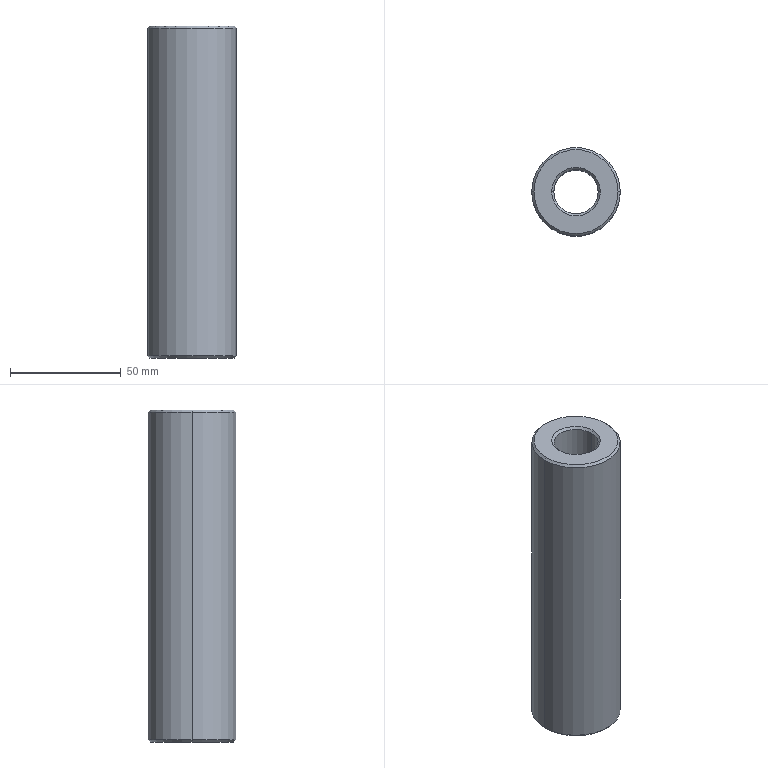Part | STEP file | BCC3 H17_2 | 1 solid | 14 faces | box 40 x 40 x 150 mm | volume 141183 mm3 | cone 8 | cylinder 4 | plane 2 | commonest cylinder face diameters 20 x2 40 x2
STEP:
#1=CARTESIAN_POINT('',(0.,0.,0.));
#2=DIRECTION('',(0.,0.,1.));
#3=DIRECTION('',(1.,0.,0.));
#4=AXIS2_PLACEMENT_3D('',#1,#2,#3);
#5=CARTESIAN_POINT('',(10.,0.,74.));
#6=VERTEX_POINT('',#5);
#7=CARTESIAN_POINT('',(11.,0.,75.));
#8=VERTEX_POINT('',#7);
#9=CARTESIAN_POINT('',(10.,0.,74.));
#10=DIRECTION('',(0.7071,0.,0.7071));
#11=VECTOR('',#10,1.);
#12=LINE('',#9,#11);
#13=CARTESIAN_POINT('',(0.,0.,74.));
#14=DIRECTION('',(0.,0.,1.));
#15=DIRECTION('',(1.,0.,0.));
#16=AXIS2_PLACEMENT_3D('',#13,#14,#15);
#17=CONICAL_SURFACE('',#16,10.,0.7854);
#18=CARTESIAN_POINT('',(6.283,0.));
#19=DIRECTION('',(0.,1.));
#20=VECTOR('',#19,1.);
#21=LINE('',#18,#20);
#22=(GEOMETRIC_REPRESENTATION_CONTEXT(2)PARAMETRIC_REPRESENTATION_CONTEXT()REPRESENTATION_CONTEXT('',''));
#23=DEFINITIONAL_REPRESENTATION('',(#21),#22);
#24=PCURVE('',#17,#23);
#25=CARTESIAN_POINT('',(0.,0.,74.));
#26=DIRECTION('',(0.,0.,1.));
#27=DIRECTION('',(1.,0.,0.));
#28=AXIS2_PLACEMENT_3D('',#25,#26,#27);
#29=CONICAL_SURFACE('',#28,10.,0.7854);
#30=CARTESIAN_POINT('',(0.,0.));
#31=DIRECTION('',(0.,1.));
#32=VECTOR('',#31,1.);
#33=LINE('',#30,#32);
#34=(GEOMETRIC_REPRESENTATION_CONTEXT(2)PARAMETRIC_REPRESENTATION_CONTEXT()REPRESENTATION_CONTEXT('',''));
#35=DEFINITIONAL_REPRESENTATION('',(#33),#34);
#36=PCURVE('',#29,#35);
#37=SURFACE_CURVE('',#12,(#24,#36),.PCURVE_S1.);
#38=EDGE_CURVE('',#6,#8,#37,.T.);
#39=ORIENTED_EDGE('',*,*,#38,.T.);
#40=CARTESIAN_POINT('',(-11.,0.,75.));
#41=VERTEX_POINT('',#40);
#42=CARTESIAN_POINT('',(0.,0.,75.));
#43=DIRECTION('',(0.,0.,-1.));
#44=DIRECTION('',(1.,0.,0.));
#45=AXIS2_PLACEMENT_3D('',#42,#43,#44);
#46=CIRCLE('',#45,11.);
#47=CARTESIAN_POINT('',(6.283,1.));
#48=DIRECTION('',(-1.,0.));
#49=VECTOR('',#48,1.);
#50=LINE('',#47,#49);
#51=(GEOMETRIC_REPRESENTATION_CONTEXT(2)PARAMETRIC_REPRESENTATION_CONTEXT()REPRESENTATION_CONTEXT('',''));
#52=DEFINITIONAL_REPRESENTATION('',(#50),#51);
#53=PCURVE('',#17,#52);
#54=CARTESIAN_POINT('',(0.,0.,75.));
#55=DIRECTION('',(0.,0.,1.));
#56=DIRECTION('',(1.,0.,0.));
#57=AXIS2_PLACEMENT_3D('',#54,#55,#56);
#58=PLANE('',#57);
#59=CARTESIAN_POINT('',(11.,0.));
#60=CARTESIAN_POINT('',(11.,-19.053));
#61=CARTESIAN_POINT('',(-5.5,-9.526));
#62=CARTESIAN_POINT('',(-22.,0.));
#63=CARTESIAN_POINT('',(-5.5,9.526));
#64=CARTESIAN_POINT('',(11.,19.053));
#65=CARTESIAN_POINT('',(11.,0.));
#66=(BOUNDED_CURVE()B_SPLINE_CURVE(2,(#59,#60,#61,#62,#63,#64,#65),.UNSPECIFIED.,.T.,.F.)B_SPLINE_CURVE_WITH_KNOTS((1,2,2,2,2,1),(-2.094,0.,2.094,4.189,6.283,8.378),.UNSPECIFIED.)CURVE()GEOMETRIC_REPRESENTATION_ITEM()RATIONAL_B_SPLINE_CURVE((1.,0.5,1.,0.5,1.,0.5,1.))REPRESENTATION_ITEM(''));
#67=(GEOMETRIC_REPRESENTATION_CONTEXT(2)PARAMETRIC_REPRESENTATION_CONTEXT()REPRESENTATION_CONTEXT('',''));
#68=DEFINITIONAL_REPRESENTATION('',(#66),#67);
#69=PCURVE('',#58,#68);
#70=SURFACE_CURVE('',#46,(#53,#69),.PCURVE_S1.);
#71=EDGE_CURVE('',#8,#41,#70,.T.);
#72=ORIENTED_EDGE('',*,*,#71,.T.);
#73=CARTESIAN_POINT('',(-10.,0.,74.));
#74=VERTEX_POINT('',#73);
#75=CARTESIAN_POINT('',(-10.,0.,74.));
#76=DIRECTION('',(-0.7071,0.,0.7071));
#77=VECTOR('',#76,1.);
#78=LINE('',#75,#77);
#79=CARTESIAN_POINT('',(3.142,0.));
#80=DIRECTION('',(0.,1.));
#81=VECTOR('',#80,1.);
#82=LINE('',#79,#81);
#83=(GEOMETRIC_REPRESENTATION_CONTEXT(2)PARAMETRIC_REPRESENTATION_CONTEXT()REPRESENTATION_CONTEXT('',''));
#84=DEFINITIONAL_REPRESENTATION('',(#82),#83);
#85=PCURVE('',#17,#84);
#86=CARTESIAN_POINT('',(3.142,0.));
#87=DIRECTION('',(0.,1.));
#88=VECTOR('',#87,1.);
#89=LINE('',#86,#88);
#90=(GEOMETRIC_REPRESENTATION_CONTEXT(2)PARAMETRIC_REPRESENTATION_CONTEXT()REPRESENTATION_CONTEXT('',''));
#91=DEFINITIONAL_REPRESENTATION('',(#89),#90);
#92=PCURVE('',#29,#91);
#93=SURFACE_CURVE('',#78,(#85,#92),.PCURVE_S1.);
#94=EDGE_CURVE('',#74,#41,#93,.T.);
#95=ORIENTED_EDGE('',*,*,#94,.F.);
#96=CARTESIAN_POINT('',(0.,0.,74.));
#97=DIRECTION('',(0.,0.,1.));
#98=DIRECTION('',(1.,0.,0.));
#99=AXIS2_PLACEMENT_3D('',#96,#97,#98);
#100=CIRCLE('',#99,10.);
#101=CARTESIAN_POINT('',(0.,0.));
#102=DIRECTION('',(1.,0.));
#103=VECTOR('',#102,1.);
#104=LINE('',#101,#103);
#105=(GEOMETRIC_REPRESENTATION_CONTEXT(2)PARAMETRIC_REPRESENTATION_CONTEXT()REPRESENTATION_CONTEXT('',''));
#106=DEFINITIONAL_REPRESENTATION('',(#104),#105);
#107=PCURVE('',#17,#106);
#108=CARTESIAN_POINT('',(0.,0.,75.));
#109=DIRECTION('',(0.,0.,-1.));
#110=DIRECTION('',(-1.,0.,0.));
#111=AXIS2_PLACEMENT_3D('',#108,#109,#110);
#112=CYLINDRICAL_SURFACE('',#111,10.);
#113=CARTESIAN_POINT('',(9.425,1.));
#114=DIRECTION('',(-1.,0.));
#115=VECTOR('',#114,1.);
#116=LINE('',#113,#115);
#117=(GEOMETRIC_REPRESENTATION_CONTEXT(2)PARAMETRIC_REPRESENTATION_CONTEXT()REPRESENTATION_CONTEXT('',''));
#118=DEFINITIONAL_REPRESENTATION('',(#116),#117);
#119=PCURVE('',#112,#118);
#120=SURFACE_CURVE('',#100,(#107,#119),.PCURVE_S1.);
#121=EDGE_CURVE('',#74,#6,#120,.T.);
#122=ORIENTED_EDGE('',*,*,#121,.T.);
#123=EDGE_LOOP('',(#39,#72,#95,#122));
#124=FACE_BOUND('',#123,.F.);
#125=ADVANCED_FACE('',(#124),#17,.F.);
#126=CARTESIAN_POINT('',(19.,0.,75.));
#127=VERTEX_POINT('',#126);
#128=CARTESIAN_POINT('',(-19.,0.,75.));
#129=VERTEX_POINT('',#128);
#130=CARTESIAN_POINT('',(0.,0.,75.));
#131=DIRECTION('',(0.,0.,1.));
#132=DIRECTION('',(1.,0.,0.));
#133=AXIS2_PLACEMENT_3D('',#130,#131,#132);
#134=CIRCLE('',#133,19.);
#135=CARTESIAN_POINT('',(0.,0.,75.));
#136=DIRECTION('',(0.,0.,-1.));
#137=DIRECTION('',(-1.,0.,0.));
#138=AXIS2_PLACEMENT_3D('',#135,#136,#137);
#139=CONICAL_SURFACE('',#138,19.,0.7854);
#140=CARTESIAN_POINT('',(3.142,0.));
#141=DIRECTION('',(-1.,0.));
#142=VECTOR('',#141,1.);
#143=LINE('',#140,#142);
#144=(GEOMETRIC_REPRESENTATION_CONTEXT(2)PARAMETRIC_REPRESENTATION_CONTEXT()REPRESENTATION_CONTEXT('',''));
#145=DEFINITIONAL_REPRESENTATION('',(#143),#144);
#146=PCURVE('',#139,#145);
#147=CARTESIAN_POINT('',(0.,0.));
#148=DIRECTION('',(1.,0.));
#149=AXIS2_PLACEMENT_2D('',#147,#148);
#150=CIRCLE('',#149,19.);
#151=(GEOMETRIC_REPRESENTATION_CONTEXT(2)PARAMETRIC_REPRESENTATION_CONTEXT()REPRESENTATION_CONTEXT('',''));
#152=DEFINITIONAL_REPRESENTATION('',(#150),#151);
#153=PCURVE('',#58,#152);
#154=SURFACE_CURVE('',#134,(#146,#153),.PCURVE_S1.);
#155=EDGE_CURVE('',#127,#129,#154,.T.);
#156=ORIENTED_EDGE('',*,*,#155,.F.);
#157=CARTESIAN_POINT('',(20.,0.,74.));
#158=VERTEX_POINT('',#157);
#159=CARTESIAN_POINT('',(19.,0.,75.));
#160=DIRECTION('',(0.7071,0.,-0.7071));
#161=VECTOR('',#160,1.);
#162=LINE('',#159,#161);
#163=CARTESIAN_POINT('',(3.142,0.));
#164=DIRECTION('',(0.,1.));
#165=VECTOR('',#164,1.);
#166=LINE('',#163,#165);
#167=(GEOMETRIC_REPRESENTATION_CONTEXT(2)PARAMETRIC_REPRESENTATION_CONTEXT()REPRESENTATION_CONTEXT('',''));
#168=DEFINITIONAL_REPRESENTATION('',(#166),#167);
#169=PCURVE('',#139,#168);
#170=CARTESIAN_POINT('',(0.,0.,75.));
#171=DIRECTION('',(0.,0.,-1.));
#172=DIRECTION('',(-1.,0.,0.));
#173=AXIS2_PLACEMENT_3D('',#170,#171,#172);
#174=CONICAL_SURFACE('',#173,19.,0.7854);
#175=CARTESIAN_POINT('',(3.142,0.));
#176=DIRECTION('',(0.,1.));
#177=VECTOR('',#176,1.);
#178=LINE('',#175,#177);
#179=(GEOMETRIC_REPRESENTATION_CONTEXT(2)PARAMETRIC_REPRESENTATION_CONTEXT()REPRESENTATION_CONTEXT('',''));
#180=DEFINITIONAL_REPRESENTATION('',(#178),#179);
#181=PCURVE('',#174,#180);
#182=SURFACE_CURVE('',#162,(#169,#181),.PCURVE_S1.);
#183=EDGE_CURVE('',#127,#158,#182,.T.);
#184=ORIENTED_EDGE('',*,*,#183,.T.);
#185=CARTESIAN_POINT('',(-20.,0.,74.));
#186=VERTEX_POINT('',#185);
#187=CARTESIAN_POINT('',(0.,0.,74.));
#188=DIRECTION('',(0.,0.,-1.));
#189=DIRECTION('',(1.,0.,0.));
#190=AXIS2_PLACEMENT_3D('',#187,#188,#189);
#191=CIRCLE('',#190,20.);
#192=CARTESIAN_POINT('',(-3.142,1.));
#193=DIRECTION('',(1.,0.));
#194=VECTOR('',#193,1.);
#195=LINE('',#192,#194);
#196=(GEOMETRIC_REPRESENTATION_CONTEXT(2)PARAMETRIC_REPRESENTATION_CONTEXT()REPRESENTATION_CONTEXT('',''));
#197=DEFINITIONAL_REPRESENTATION('',(#195),#196);
#198=PCURVE('',#139,#197);
#199=CARTESIAN_POINT('',(0.,0.,75.));
#200=DIRECTION('',(0.,0.,-1.));
#201=DIRECTION('',(-1.,0.,0.));
#202=AXIS2_PLACEMENT_3D('',#199,#200,#201);
#203=CYLINDRICAL_SURFACE('',#202,20.);
#204=CARTESIAN_POINT('',(-3.142,1.));
#205=DIRECTION('',(1.,0.));
#206=VECTOR('',#205,1.);
#207=LINE('',#204,#206);
#208=(GEOMETRIC_REPRESENTATION_CONTEXT(2)PARAMETRIC_REPRESENTATION_CONTEXT()REPRESENTATION_CONTEXT('',''));
#209=DEFINITIONAL_REPRESENTATION('',(#207),#208);
#210=PCURVE('',#203,#209);
#211=SURFACE_CURVE('',#191,(#198,#210),.PCURVE_S1.);
#212=EDGE_CURVE('',#186,#158,#211,.T.);
#213=ORIENTED_EDGE('',*,*,#212,.F.);
#214=CARTESIAN_POINT('',(-19.,0.,75.));
#215=DIRECTION('',(-0.7071,0.,-0.7071));
#216=VECTOR('',#215,1.);
#217=LINE('',#214,#216);
#218=CARTESIAN_POINT('',(0.,0.));
#219=DIRECTION('',(0.,1.));
#220=VECTOR('',#219,1.);
#221=LINE('',#218,#220);
#222=(GEOMETRIC_REPRESENTATION_CONTEXT(2)PARAMETRIC_REPRESENTATION_CONTEXT()REPRESENTATION_CONTEXT('',''));
#223=DEFINITIONAL_REPRESENTATION('',(#221),#222);
#224=PCURVE('',#139,#223);
#225=CARTESIAN_POINT('',(6.283,0.));
#226=DIRECTION('',(0.,1.));
#227=VECTOR('',#226,1.);
#228=LINE('',#225,#227);
#229=(GEOMETRIC_REPRESENTATION_CONTEXT(2)PARAMETRIC_REPRESENTATION_CONTEXT()REPRESENTATION_CONTEXT('',''));
#230=DEFINITIONAL_REPRESENTATION('',(#228),#229);
#231=PCURVE('',#174,#230);
#232=SURFACE_CURVE('',#217,(#224,#231),.PCURVE_S1.);
#233=EDGE_CURVE('',#129,#186,#232,.T.);
#234=ORIENTED_EDGE('',*,*,#233,.F.);
#235=EDGE_LOOP('',(#156,#184,#213,#234));
#236=FACE_BOUND('',#235,.T.);
#237=ADVANCED_FACE('',(#236),#139,.T.);
#238=CARTESIAN_POINT('',(-19.,0.,-75.));
#239=VERTEX_POINT('',#238);
#240=CARTESIAN_POINT('',(19.,0.,-75.));
#241=VERTEX_POINT('',#240);
#242=CARTESIAN_POINT('',(0.,0.,-75.));
#243=DIRECTION('',(0.,0.,-1.));
#244=DIRECTION('',(1.,0.,0.));
#245=AXIS2_PLACEMENT_3D('',#242,#243,#244);
#246=CIRCLE('',#245,19.);
#247=CARTESIAN_POINT('',(0.,0.,-74.));
#248=DIRECTION('',(0.,0.,1.));
#249=DIRECTION('',(1.,0.,0.));
#250=AXIS2_PLACEMENT_3D('',#247,#248,#249);
#251=CONICAL_SURFACE('',#250,20.,0.7854);
#252=CARTESIAN_POINT('',(6.283,-1.));
#253=DIRECTION('',(-1.,0.));
#254=VECTOR('',#253,1.);
#255=LINE('',#252,#254);
#256=(GEOMETRIC_REPRESENTATION_CONTEXT(2)PARAMETRIC_REPRESENTATION_CONTEXT()REPRESENTATION_CONTEXT('',''));
#257=DEFINITIONAL_REPRESENTATION('',(#255),#256);
#258=PCURVE('',#251,#257);
#259=CARTESIAN_POINT('',(0.,0.,-75.));
#260=DIRECTION('',(0.,0.,1.));
#261=DIRECTION('',(1.,0.,0.));
#262=AXIS2_PLACEMENT_3D('',#259,#260,#261);
#263=PLANE('',#262);
#264=CARTESIAN_POINT('',(19.,0.));
#265=CARTESIAN_POINT('',(19.,-32.909));
#266=CARTESIAN_POINT('',(-9.5,-16.454));
#267=CARTESIAN_POINT('',(-38.,0.));
#268=CARTESIAN_POINT('',(-9.5,16.454));
#269=CARTESIAN_POINT('',(19.,32.909));
#270=CARTESIAN_POINT('',(19.,0.));
#271=(BOUNDED_CURVE()B_SPLINE_CURVE(2,(#264,#265,#266,#267,#268,#269,#270),.UNSPECIFIED.,.T.,.F.)B_SPLINE_CURVE_WITH_KNOTS((1,2,2,2,2,1),(-2.094,0.,2.094,4.189,6.283,8.378),.UNSPECIFIED.)CURVE()GEOMETRIC_REPRESENTATION_ITEM()RATIONAL_B_SPLINE_CURVE((1.,0.5,1.,0.5,1.,0.5,1.))REPRESENTATION_ITEM(''));
#272=(GEOMETRIC_REPRESENTATION_CONTEXT(2)PARAMETRIC_REPRESENTATION_CONTEXT()REPRESENTATION_CONTEXT('',''));
#273=DEFINITIONAL_REPRESENTATION('',(#271),#272);
#274=PCURVE('',#263,#273);
#275=SURFACE_CURVE('',#246,(#258,#274),.PCURVE_S1.);
#276=EDGE_CURVE('',#239,#241,#275,.T.);
#277=ORIENTED_EDGE('',*,*,#276,.F.);
#278=CARTESIAN_POINT('',(-20.,0.,-74.));
#279=VERTEX_POINT('',#278);
#280=CARTESIAN_POINT('',(-20.,0.,-74.));
#281=DIRECTION('',(-0.7071,0.,0.7071));
#282=VECTOR('',#281,1.);
#283=LINE('',#280,#282);
#284=CARTESIAN_POINT('',(3.142,0.));
#285=DIRECTION('',(0.,1.));
#286=VECTOR('',#285,1.);
#287=LINE('',#284,#286);
#288=(GEOMETRIC_REPRESENTATION_CONTEXT(2)PARAMETRIC_REPRESENTATION_CONTEXT()REPRESENTATION_CONTEXT('',''));
#289=DEFINITIONAL_REPRESENTATION('',(#287),#288);
#290=PCURVE('',#251,#289);
#291=CARTESIAN_POINT('',(0.,0.,-74.));
#292=DIRECTION('',(0.,0.,1.));
#293=DIRECTION('',(1.,0.,0.));
#294=AXIS2_PLACEMENT_3D('',#291,#292,#293);
#295=CONICAL_SURFACE('',#294,20.,0.7854);
#296=CARTESIAN_POINT('',(3.142,0.));
#297=DIRECTION('',(0.,1.));
#298=VECTOR('',#297,1.);
#299=LINE('',#296,#298);
#300=(GEOMETRIC_REPRESENTATION_CONTEXT(2)PARAMETRIC_REPRESENTATION_CONTEXT()REPRESENTATION_CONTEXT('',''));
#301=DEFINITIONAL_REPRESENTATION('',(#299),#300);
#302=PCURVE('',#295,#301);
#303=SURFACE_CURVE('',#283,(#290,#302),.PCURVE_S1.);
#304=EDGE_CURVE('',#239,#279,#303,.T.);
#305=ORIENTED_EDGE('',*,*,#304,.T.);
#306=CARTESIAN_POINT('',(20.,0.,-74.));
#307=VERTEX_POINT('',#306);
#308=CARTESIAN_POINT('',(0.,0.,-74.));
#309=DIRECTION('',(0.,0.,1.));
#310=DIRECTION('',(1.,0.,0.));
#311=AXIS2_PLACEMENT_3D('',#308,#309,#310);
#312=CIRCLE('',#311,20.);
#313=CARTESIAN_POINT('',(0.,0.));
#314=DIRECTION('',(1.,0.));
#315=VECTOR('',#314,1.);
#316=LINE('',#313,#315);
#317=(GEOMETRIC_REPRESENTATION_CONTEXT(2)PARAMETRIC_REPRESENTATION_CONTEXT()REPRESENTATION_CONTEXT('',''));
#318=DEFINITIONAL_REPRESENTATION('',(#316),#317);
#319=PCURVE('',#251,#318);
#320=CARTESIAN_POINT('',(3.142,149.));
#321=DIRECTION('',(-1.,0.));
#322=VECTOR('',#321,1.);
#323=LINE('',#320,#322);
#324=(GEOMETRIC_REPRESENTATION_CONTEXT(2)PARAMETRIC_REPRESENTATION_CONTEXT()REPRESENTATION_CONTEXT('',''));
#325=DEFINITIONAL_REPRESENTATION('',(#323),#324);
#326=PCURVE('',#203,#325);
#327=SURFACE_CURVE('',#312,(#319,#326),.PCURVE_S1.);
#328=EDGE_CURVE('',#307,#279,#327,.T.);
#329=ORIENTED_EDGE('',*,*,#328,.F.);
#330=CARTESIAN_POINT('',(20.,0.,-74.));
#331=DIRECTION('',(0.7071,0.,0.7071));
#332=VECTOR('',#331,1.);
#333=LINE('',#330,#332);
#334=CARTESIAN_POINT('',(0.,0.));
#335=DIRECTION('',(0.,1.));
#336=VECTOR('',#335,1.);
#337=LINE('',#334,#336);
#338=(GEOMETRIC_REPRESENTATION_CONTEXT(2)PARAMETRIC_REPRESENTATION_CONTEXT()REPRESENTATION_CONTEXT('',''));
#339=DEFINITIONAL_REPRESENTATION('',(#337),#338);
#340=PCURVE('',#251,#339);
#341=CARTESIAN_POINT('',(6.283,0.));
#342=DIRECTION('',(0.,1.));
#343=VECTOR('',#342,1.);
#344=LINE('',#341,#343);
#345=(GEOMETRIC_REPRESENTATION_CONTEXT(2)PARAMETRIC_REPRESENTATION_CONTEXT()REPRESENTATION_CONTEXT('',''));
#346=DEFINITIONAL_REPRESENTATION('',(#344),#345);
#347=PCURVE('',#295,#346);
#348=SURFACE_CURVE('',#333,(#340,#347),.PCURVE_S1.);
#349=EDGE_CURVE('',#241,#307,#348,.T.);
#350=ORIENTED_EDGE('',*,*,#349,.F.);
#351=EDGE_LOOP('',(#277,#305,#329,#350));
#352=FACE_BOUND('',#351,.T.);
#353=ADVANCED_FACE('',(#352),#251,.T.);
#354=CARTESIAN_POINT('',(-10.,0.,-74.));
#355=VERTEX_POINT('',#354);
#356=CARTESIAN_POINT('',(-11.,0.,-75.));
#357=VERTEX_POINT('',#356);
#358=CARTESIAN_POINT('',(-11.,0.,-75.));
#359=DIRECTION('',(-0.7071,0.,-0.7071));
#360=VECTOR('',#359,1.);
#361=LINE('',#358,#360);
#362=CARTESIAN_POINT('',(0.,0.,-75.));
#363=DIRECTION('',(0.,0.,-1.));
#364=DIRECTION('',(-1.,0.,0.));
#365=AXIS2_PLACEMENT_3D('',#362,#363,#364);
#366=CONICAL_SURFACE('',#365,11.,0.7854);
#367=CARTESIAN_POINT('',(6.283,0.));
#368=DIRECTION('',(0.,1.));
#369=VECTOR('',#368,1.);
#370=LINE('',#367,#369);
#371=(GEOMETRIC_REPRESENTATION_CONTEXT(2)PARAMETRIC_REPRESENTATION_CONTEXT()REPRESENTATION_CONTEXT('',''));
#372=DEFINITIONAL_REPRESENTATION('',(#370),#371);
#373=PCURVE('',#366,#372);
#374=CARTESIAN_POINT('',(0.,0.,-75.));
#375=DIRECTION('',(0.,0.,-1.));
#376=DIRECTION('',(-1.,0.,0.));
#377=AXIS2_PLACEMENT_3D('',#374,#375,#376);
#378=CONICAL_SURFACE('',#377,11.,0.7854);
#379=CARTESIAN_POINT('',(0.,0.));
#380=DIRECTION('',(0.,1.));
#381=VECTOR('',#380,1.);
#382=LINE('',#379,#381);
#383=(GEOMETRIC_REPRESENTATION_CONTEXT(2)PARAMETRIC_REPRESENTATION_CONTEXT()REPRESENTATION_CONTEXT('',''));
#384=DEFINITIONAL_REPRESENTATION('',(#382),#383);
#385=PCURVE('',#378,#384);
#386=SURFACE_CURVE('',#361,(#373,#385),.PCURVE_S1.);
#387=EDGE_CURVE('',#355,#357,#386,.T.);
#388=ORIENTED_EDGE('',*,*,#387,.T.);
#389=CARTESIAN_POINT('',(11.,0.,-75.));
#390=VERTEX_POINT('',#389);
#391=CARTESIAN_POINT('',(0.,0.,-75.));
#392=DIRECTION('',(0.,0.,1.));
#393=DIRECTION('',(1.,0.,0.));
#394=AXIS2_PLACEMENT_3D('',#391,#392,#393);
#395=CIRCLE('',#394,11.);
#396=CARTESIAN_POINT('',(9.425,0.));
#397=DIRECTION('',(-1.,0.));
#398=VECTOR('',#397,1.);
#399=LINE('',#396,#398);
#400=(GEOMETRIC_REPRESENTATION_CONTEXT(2)PARAMETRIC_REPRESENTATION_CONTEXT()REPRESENTATION_CONTEXT('',''));
#401=DEFINITIONAL_REPRESENTATION('',(#399),#400);
#402=PCURVE('',#366,#401);
#403=CARTESIAN_POINT('',(0.,0.));
#404=DIRECTION('',(1.,0.));
#405=AXIS2_PLACEMENT_2D('',#403,#404);
#406=CIRCLE('',#405,11.);
#407=(GEOMETRIC_REPRESENTATION_CONTEXT(2)PARAMETRIC_REPRESENTATION_CONTEXT()REPRESENTATION_CONTEXT('',''));
#408=DEFINITIONAL_REPRESENTATION('',(#406),#407);
#409=PCURVE('',#263,#408);
#410=SURFACE_CURVE('',#395,(#402,#409),.PCURVE_S1.);
#411=EDGE_CURVE('',#357,#390,#410,.T.);
#412=ORIENTED_EDGE('',*,*,#411,.T.);
#413=CARTESIAN_POINT('',(10.,0.,-74.));
#414=VERTEX_POINT('',#413);
#415=CARTESIAN_POINT('',(11.,0.,-75.));
#416=DIRECTION('',(0.7071,0.,-0.7071));
#417=VECTOR('',#416,1.);
#418=LINE('',#415,#417);
#419=CARTESIAN_POINT('',(3.142,0.));
#420=DIRECTION('',(0.,1.));
#421=VECTOR('',#420,1.);
#422=LINE('',#419,#421);
#423=(GEOMETRIC_REPRESENTATION_CONTEXT(2)PARAMETRIC_REPRESENTATION_CONTEXT()REPRESENTATION_CONTEXT('',''));
#424=DEFINITIONAL_REPRESENTATION('',(#422),#423);
#425=PCURVE('',#366,#424);
#426=CARTESIAN_POINT('',(3.142,0.));
#427=DIRECTION('',(0.,1.));
#428=VECTOR('',#427,1.);
#429=LINE('',#426,#428);
#430=(GEOMETRIC_REPRESENTATION_CONTEXT(2)PARAMETRIC_REPRESENTATION_CONTEXT()REPRESENTATION_CONTEXT('',''));
#431=DEFINITIONAL_REPRESENTATION('',(#429),#430);
#432=PCURVE('',#378,#431);
#433=SURFACE_CURVE('',#418,(#425,#432),.PCURVE_S1.);
#434=EDGE_CURVE('',#414,#390,#433,.T.);
#435=ORIENTED_EDGE('',*,*,#434,.F.);
#436=CARTESIAN_POINT('',(0.,0.,-74.));
#437=DIRECTION('',(0.,0.,-1.));
#438=DIRECTION('',(1.,0.,0.));
#439=AXIS2_PLACEMENT_3D('',#436,#437,#438);
#440=CIRCLE('',#439,10.);
#441=CARTESIAN_POINT('',(3.142,-1.));
#442=DIRECTION('',(1.,0.));
#443=VECTOR('',#442,1.);
#444=LINE('',#441,#443);
#445=(GEOMETRIC_REPRESENTATION_CONTEXT(2)PARAMETRIC_REPRESENTATION_CONTEXT()REPRESENTATION_CONTEXT('',''));
#446=DEFINITIONAL_REPRESENTATION('',(#444),#445);
#447=PCURVE('',#366,#446);
#448=CARTESIAN_POINT('',(3.142,149.));
#449=DIRECTION('',(1.,0.));
#450=VECTOR('',#449,1.);
#451=LINE('',#448,#450);
#452=(GEOMETRIC_REPRESENTATION_CONTEXT(2)PARAMETRIC_REPRESENTATION_CONTEXT()REPRESENTATION_CONTEXT('',''));
#453=DEFINITIONAL_REPRESENTATION('',(#451),#452);
#454=PCURVE('',#112,#453);
#455=SURFACE_CURVE('',#440,(#447,#454),.PCURVE_S1.);
#456=EDGE_CURVE('',#414,#355,#455,.T.);
#457=ORIENTED_EDGE('',*,*,#456,.T.);
#458=EDGE_LOOP('',(#388,#412,#435,#457));
#459=FACE_BOUND('',#458,.F.);
#460=ADVANCED_FACE('',(#459),#366,.F.);
#461=CARTESIAN_POINT('',(-10.,0.,75.));
#462=DIRECTION('',(0.,0.,-1.));
#463=VECTOR('',#462,1.);
#464=LINE('',#461,#463);
#465=CARTESIAN_POINT('',(6.283,0.));
#466=DIRECTION('',(0.,1.));
#467=VECTOR('',#466,1.);
#468=LINE('',#465,#467);
#469=(GEOMETRIC_REPRESENTATION_CONTEXT(2)PARAMETRIC_REPRESENTATION_CONTEXT()REPRESENTATION_CONTEXT('',''));
#470=DEFINITIONAL_REPRESENTATION('',(#468),#469);
#471=PCURVE('',#112,#470);
#472=CARTESIAN_POINT('',(0.,0.,75.));
#473=DIRECTION('',(0.,0.,-1.));
#474=DIRECTION('',(-1.,0.,0.));
#475=AXIS2_PLACEMENT_3D('',#472,#473,#474);
#476=CYLINDRICAL_SURFACE('',#475,10.);
#477=CARTESIAN_POINT('',(0.,0.));
#478=DIRECTION('',(0.,1.));
#479=VECTOR('',#478,1.);
#480=LINE('',#477,#479);
#481=(GEOMETRIC_REPRESENTATION_CONTEXT(2)PARAMETRIC_REPRESENTATION_CONTEXT()REPRESENTATION_CONTEXT('',''));
#482=DEFINITIONAL_REPRESENTATION('',(#480),#481);
#483=PCURVE('',#476,#482);
#484=SURFACE_CURVE('',#464,(#471,#483),.PCURVE_S1.);
#485=EDGE_CURVE('',#74,#355,#484,.T.);
#486=ORIENTED_EDGE('',*,*,#485,.T.);
#487=ORIENTED_EDGE('',*,*,#456,.F.);
#488=CARTESIAN_POINT('',(10.,0.,75.));
#489=DIRECTION('',(0.,0.,-1.));
#490=VECTOR('',#489,1.);
#491=LINE('',#488,#490);
#492=CARTESIAN_POINT('',(3.142,0.));
#493=DIRECTION('',(0.,1.));
#494=VECTOR('',#493,1.);
#495=LINE('',#492,#494);
#496=(GEOMETRIC_REPRESENTATION_CONTEXT(2)PARAMETRIC_REPRESENTATION_CONTEXT()REPRESENTATION_CONTEXT('',''));
#497=DEFINITIONAL_REPRESENTATION('',(#495),#496);
#498=PCURVE('',#112,#497);
#499=CARTESIAN_POINT('',(3.142,0.));
#500=DIRECTION('',(0.,1.));
#501=VECTOR('',#500,1.);
#502=LINE('',#499,#501);
#503=(GEOMETRIC_REPRESENTATION_CONTEXT(2)PARAMETRIC_REPRESENTATION_CONTEXT()REPRESENTATION_CONTEXT('',''));
#504=DEFINITIONAL_REPRESENTATION('',(#502),#503);
#505=PCURVE('',#476,#504);
#506=SURFACE_CURVE('',#491,(#498,#505),.PCURVE_S1.);
#507=EDGE_CURVE('',#6,#414,#506,.T.);
#508=ORIENTED_EDGE('',*,*,#507,.F.);
#509=ORIENTED_EDGE('',*,*,#121,.F.);
#510=EDGE_LOOP('',(#486,#487,#508,#509));
#511=FACE_BOUND('',#510,.F.);
#512=ADVANCED_FACE('',(#511),#112,.F.);
#513=ORIENTED_EDGE('',*,*,#212,.T.);
#514=CARTESIAN_POINT('',(20.,0.,75.));
#515=DIRECTION('',(0.,0.,-1.));
#516=VECTOR('',#515,1.);
#517=LINE('',#514,#516);
#518=CARTESIAN_POINT('',(3.142,0.));
#519=DIRECTION('',(0.,1.));
#520=VECTOR('',#519,1.);
#521=LINE('',#518,#520);
#522=(GEOMETRIC_REPRESENTATION_CONTEXT(2)PARAMETRIC_REPRESENTATION_CONTEXT()REPRESENTATION_CONTEXT('',''));
#523=DEFINITIONAL_REPRESENTATION('',(#521),#522);
#524=PCURVE('',#203,#523);
#525=CARTESIAN_POINT('',(0.,0.,75.));
#526=DIRECTION('',(0.,0.,-1.));
#527=DIRECTION('',(-1.,0.,0.));
#528=AXIS2_PLACEMENT_3D('',#525,#526,#527);
#529=CYLINDRICAL_SURFACE('',#528,20.);
#530=CARTESIAN_POINT('',(3.142,0.));
#531=DIRECTION('',(0.,1.));
#532=VECTOR('',#531,1.);
#533=LINE('',#530,#532);
#534=(GEOMETRIC_REPRESENTATION_CONTEXT(2)PARAMETRIC_REPRESENTATION_CONTEXT()REPRESENTATION_CONTEXT('',''));
#535=DEFINITIONAL_REPRESENTATION('',(#533),#534);
#536=PCURVE('',#529,#535);
#537=SURFACE_CURVE('',#517,(#524,#536),.PCURVE_S1.);
#538=EDGE_CURVE('',#158,#307,#537,.T.);
#539=ORIENTED_EDGE('',*,*,#538,.T.);
#540=ORIENTED_EDGE('',*,*,#328,.T.);
#541=CARTESIAN_POINT('',(-20.,0.,75.));
#542=DIRECTION('',(0.,0.,-1.));
#543=VECTOR('',#542,1.);
#544=LINE('',#541,#543);
#545=CARTESIAN_POINT('',(0.,0.));
#546=DIRECTION('',(0.,1.));
#547=VECTOR('',#546,1.);
#548=LINE('',#545,#547);
#549=(GEOMETRIC_REPRESENTATION_CONTEXT(2)PARAMETRIC_REPRESENTATION_CONTEXT()REPRESENTATION_CONTEXT('',''));
#550=DEFINITIONAL_REPRESENTATION('',(#548),#549);
#551=PCURVE('',#203,#550);
#552=CARTESIAN_POINT('',(6.283,0.));
#553=DIRECTION('',(0.,1.));
#554=VECTOR('',#553,1.);
#555=LINE('',#552,#554);
#556=(GEOMETRIC_REPRESENTATION_CONTEXT(2)PARAMETRIC_REPRESENTATION_CONTEXT()REPRESENTATION_CONTEXT('',''));
#557=DEFINITIONAL_REPRESENTATION('',(#555),#556);
#558=PCURVE('',#529,#557);
#559=SURFACE_CURVE('',#544,(#551,#558),.PCURVE_S1.);
#560=EDGE_CURVE('',#186,#279,#559,.T.);
#561=ORIENTED_EDGE('',*,*,#560,.F.);
#562=EDGE_LOOP('',(#513,#539,#540,#561));
#563=FACE_BOUND('',#562,.T.);
#564=ADVANCED_FACE('',(#563),#203,.T.);
#565=CARTESIAN_POINT('',(0.,0.,75.));
#566=DIRECTION('',(0.,0.,1.));
#567=DIRECTION('',(1.,0.,0.));
#568=AXIS2_PLACEMENT_3D('',#565,#566,#567);
#569=CIRCLE('',#568,19.);
#570=CARTESIAN_POINT('',(0.,0.));
#571=DIRECTION('',(1.,0.));
#572=AXIS2_PLACEMENT_2D('',#570,#571);
#573=CIRCLE('',#572,19.);
#574=(GEOMETRIC_REPRESENTATION_CONTEXT(2)PARAMETRIC_REPRESENTATION_CONTEXT()REPRESENTATION_CONTEXT('',''));
#575=DEFINITIONAL_REPRESENTATION('',(#573),#574);
#576=PCURVE('',#58,#575);
#577=CARTESIAN_POINT('',(9.425,0.));
#578=DIRECTION('',(-1.,0.));
#579=VECTOR('',#578,1.);
#580=LINE('',#577,#579);
#581=(GEOMETRIC_REPRESENTATION_CONTEXT(2)PARAMETRIC_REPRESENTATION_CONTEXT()REPRESENTATION_CONTEXT('',''));
#582=DEFINITIONAL_REPRESENTATION('',(#580),#581);
#583=PCURVE('',#174,#582);
#584=SURFACE_CURVE('',#569,(#576,#583),.PCURVE_S1.);
#585=EDGE_CURVE('',#129,#127,#584,.T.);
#586=ORIENTED_EDGE('',*,*,#585,.T.);
#587=ORIENTED_EDGE('',*,*,#155,.T.);
#588=EDGE_LOOP('',(#586,#587));
#589=FACE_BOUND('',#588,.T.);
#590=ORIENTED_EDGE('',*,*,#71,.T.);
#591=CARTESIAN_POINT('',(0.,0.,75.));
#592=DIRECTION('',(0.,0.,-1.));
#593=DIRECTION('',(1.,0.,0.));
#594=AXIS2_PLACEMENT_3D('',#591,#592,#593);
#595=CIRCLE('',#594,11.);
#596=CARTESIAN_POINT('',(11.,0.));
#597=CARTESIAN_POINT('',(11.,-19.053));
#598=CARTESIAN_POINT('',(-5.5,-9.526));
#599=CARTESIAN_POINT('',(-22.,0.));
#600=CARTESIAN_POINT('',(-5.5,9.526));
#601=CARTESIAN_POINT('',(11.,19.053));
#602=CARTESIAN_POINT('',(11.,0.));
#603=(BOUNDED_CURVE()B_SPLINE_CURVE(2,(#596,#597,#598,#599,#600,#601,#602),.UNSPECIFIED.,.T.,.F.)B_SPLINE_CURVE_WITH_KNOTS((1,2,2,2,2,1),(-2.094,0.,2.094,4.189,6.283,8.378),.UNSPECIFIED.)CURVE()GEOMETRIC_REPRESENTATION_ITEM()RATIONAL_B_SPLINE_CURVE((1.,0.5,1.,0.5,1.,0.5,1.))REPRESENTATION_ITEM(''));
#604=(GEOMETRIC_REPRESENTATION_CONTEXT(2)PARAMETRIC_REPRESENTATION_CONTEXT()REPRESENTATION_CONTEXT('',''));
#605=DEFINITIONAL_REPRESENTATION('',(#603),#604);
#606=PCURVE('',#58,#605);
#607=CARTESIAN_POINT('',(6.283,1.));
#608=DIRECTION('',(-1.,0.));
#609=VECTOR('',#608,1.);
#610=LINE('',#607,#609);
#611=(GEOMETRIC_REPRESENTATION_CONTEXT(2)PARAMETRIC_REPRESENTATION_CONTEXT()REPRESENTATION_CONTEXT('',''));
#612=DEFINITIONAL_REPRESENTATION('',(#610),#611);
#613=PCURVE('',#29,#612);
#614=SURFACE_CURVE('',#595,(#606,#613),.PCURVE_S1.);
#615=EDGE_CURVE('',#41,#8,#614,.T.);
#616=ORIENTED_EDGE('',*,*,#615,.T.);
#617=EDGE_LOOP('',(#590,#616));
#618=FACE_BOUND('',#617,.T.);
#619=ADVANCED_FACE('',(#589,#618),#58,.T.);
#620=ORIENTED_EDGE('',*,*,#411,.T.);
#621=CARTESIAN_POINT('',(0.,0.,-75.));
#622=DIRECTION('',(0.,0.,1.));
#623=DIRECTION('',(1.,0.,0.));
#624=AXIS2_PLACEMENT_3D('',#621,#622,#623);
#625=CIRCLE('',#624,11.);
#626=CARTESIAN_POINT('',(0.,0.));
#627=DIRECTION('',(1.,0.));
#628=AXIS2_PLACEMENT_2D('',#626,#627);
#629=CIRCLE('',#628,11.);
#630=(GEOMETRIC_REPRESENTATION_CONTEXT(2)PARAMETRIC_REPRESENTATION_CONTEXT()REPRESENTATION_CONTEXT('',''));
#631=DEFINITIONAL_REPRESENTATION('',(#629),#630);
#632=PCURVE('',#263,#631);
#633=CARTESIAN_POINT('',(3.142,0.));
#634=DIRECTION('',(-1.,0.));
#635=VECTOR('',#634,1.);
#636=LINE('',#633,#635);
#637=(GEOMETRIC_REPRESENTATION_CONTEXT(2)PARAMETRIC_REPRESENTATION_CONTEXT()REPRESENTATION_CONTEXT('',''));
#638=DEFINITIONAL_REPRESENTATION('',(#636),#637);
#639=PCURVE('',#378,#638);
#640=SURFACE_CURVE('',#625,(#632,#639),.PCURVE_S1.);
#641=EDGE_CURVE('',#390,#357,#640,.T.);
#642=ORIENTED_EDGE('',*,*,#641,.T.);
#643=EDGE_LOOP('',(#620,#642));
#644=FACE_BOUND('',#643,.T.);
#645=CARTESIAN_POINT('',(0.,0.,-75.));
#646=DIRECTION('',(0.,0.,-1.));
#647=DIRECTION('',(1.,0.,0.));
#648=AXIS2_PLACEMENT_3D('',#645,#646,#647);
#649=CIRCLE('',#648,19.);
#650=CARTESIAN_POINT('',(19.,0.));
#651=CARTESIAN_POINT('',(19.,-32.909));
#652=CARTESIAN_POINT('',(-9.5,-16.454));
#653=CARTESIAN_POINT('',(-38.,0.));
#654=CARTESIAN_POINT('',(-9.5,16.454));
#655=CARTESIAN_POINT('',(19.,32.909));
#656=CARTESIAN_POINT('',(19.,0.));
#657=(BOUNDED_CURVE()B_SPLINE_CURVE(2,(#650,#651,#652,#653,#654,#655,#656),.UNSPECIFIED.,.T.,.F.)B_SPLINE_CURVE_WITH_KNOTS((1,2,2,2,2,1),(-2.094,0.,2.094,4.189,6.283,8.378),.UNSPECIFIED.)CURVE()GEOMETRIC_REPRESENTATION_ITEM()RATIONAL_B_SPLINE_CURVE((1.,0.5,1.,0.5,1.,0.5,1.))REPRESENTATION_ITEM(''));
#658=(GEOMETRIC_REPRESENTATION_CONTEXT(2)PARAMETRIC_REPRESENTATION_CONTEXT()REPRESENTATION_CONTEXT('',''));
#659=DEFINITIONAL_REPRESENTATION('',(#657),#658);
#660=PCURVE('',#263,#659);
#661=CARTESIAN_POINT('',(6.283,-1.));
#662=DIRECTION('',(-1.,0.));
#663=VECTOR('',#662,1.);
#664=LINE('',#661,#663);
#665=(GEOMETRIC_REPRESENTATION_CONTEXT(2)PARAMETRIC_REPRESENTATION_CONTEXT()REPRESENTATION_CONTEXT('',''));
#666=DEFINITIONAL_REPRESENTATION('',(#664),#665);
#667=PCURVE('',#295,#666);
#668=SURFACE_CURVE('',#649,(#660,#667),.PCURVE_S1.);
#669=EDGE_CURVE('',#241,#239,#668,.T.);
#670=ORIENTED_EDGE('',*,*,#669,.T.);
#671=ORIENTED_EDGE('',*,*,#276,.T.);
#672=EDGE_LOOP('',(#670,#671));
#673=FACE_BOUND('',#672,.T.);
#674=ADVANCED_FACE('',(#644,#673),#263,.F.);
#675=ORIENTED_EDGE('',*,*,#538,.F.);
#676=CARTESIAN_POINT('',(0.,0.,74.));
#677=DIRECTION('',(0.,0.,-1.));
#678=DIRECTION('',(1.,0.,0.));
#679=AXIS2_PLACEMENT_3D('',#676,#677,#678);
#680=CIRCLE('',#679,20.);
#681=CARTESIAN_POINT('',(3.142,1.));
#682=DIRECTION('',(1.,0.));
#683=VECTOR('',#682,1.);
#684=LINE('',#681,#683);
#685=(GEOMETRIC_REPRESENTATION_CONTEXT(2)PARAMETRIC_REPRESENTATION_CONTEXT()REPRESENTATION_CONTEXT('',''));
#686=DEFINITIONAL_REPRESENTATION('',(#684),#685);
#687=PCURVE('',#529,#686);
#688=CARTESIAN_POINT('',(3.142,1.));
#689=DIRECTION('',(1.,0.));
#690=VECTOR('',#689,1.);
#691=LINE('',#688,#690);
#692=(GEOMETRIC_REPRESENTATION_CONTEXT(2)PARAMETRIC_REPRESENTATION_CONTEXT()REPRESENTATION_CONTEXT('',''));
#693=DEFINITIONAL_REPRESENTATION('',(#691),#692);
#694=PCURVE('',#174,#693);
#695=SURFACE_CURVE('',#680,(#687,#694),.PCURVE_S1.);
#696=EDGE_CURVE('',#158,#186,#695,.T.);
#697=ORIENTED_EDGE('',*,*,#696,.T.);
#698=ORIENTED_EDGE('',*,*,#560,.T.);
#699=CARTESIAN_POINT('',(0.,0.,-74.));
#700=DIRECTION('',(0.,0.,1.));
#701=DIRECTION('',(1.,0.,0.));
#702=AXIS2_PLACEMENT_3D('',#699,#700,#701);
#703=CIRCLE('',#702,20.);
#704=CARTESIAN_POINT('',(9.425,149.));
#705=DIRECTION('',(-1.,0.));
#706=VECTOR('',#705,1.);
#707=LINE('',#704,#706);
#708=(GEOMETRIC_REPRESENTATION_CONTEXT(2)PARAMETRIC_REPRESENTATION_CONTEXT()REPRESENTATION_CONTEXT('',''));
#709=DEFINITIONAL_REPRESENTATION('',(#707),#708);
#710=PCURVE('',#529,#709);
#711=CARTESIAN_POINT('',(0.,0.));
#712=DIRECTION('',(1.,0.));
#713=VECTOR('',#712,1.);
#714=LINE('',#711,#713);
#715=(GEOMETRIC_REPRESENTATION_CONTEXT(2)PARAMETRIC_REPRESENTATION_CONTEXT()REPRESENTATION_CONTEXT('',''));
#716=DEFINITIONAL_REPRESENTATION('',(#714),#715);
#717=PCURVE('',#295,#716);
#718=SURFACE_CURVE('',#703,(#710,#717),.PCURVE_S1.);
#719=EDGE_CURVE('',#279,#307,#718,.T.);
#720=ORIENTED_EDGE('',*,*,#719,.T.);
#721=EDGE_LOOP('',(#675,#697,#698,#720));
#722=FACE_BOUND('',#721,.T.);
#723=ADVANCED_FACE('',(#722),#529,.T.);
#724=CARTESIAN_POINT('',(0.,0.,-74.));
#725=DIRECTION('',(0.,0.,-1.));
#726=DIRECTION('',(1.,0.,0.));
#727=AXIS2_PLACEMENT_3D('',#724,#725,#726);
#728=CIRCLE('',#727,10.);
#729=CARTESIAN_POINT('',(-3.142,149.));
#730=DIRECTION('',(1.,0.));
#731=VECTOR('',#730,1.);
#732=LINE('',#729,#731);
#733=(GEOMETRIC_REPRESENTATION_CONTEXT(2)PARAMETRIC_REPRESENTATION_CONTEXT()REPRESENTATION_CONTEXT('',''));
#734=DEFINITIONAL_REPRESENTATION('',(#732),#733);
#735=PCURVE('',#476,#734);
#736=CARTESIAN_POINT('',(-3.142,-1.));
#737=DIRECTION('',(1.,0.));
#738=VECTOR('',#737,1.);
#739=LINE('',#736,#738);
#740=(GEOMETRIC_REPRESENTATION_CONTEXT(2)PARAMETRIC_REPRESENTATION_CONTEXT()REPRESENTATION_CONTEXT('',''));
#741=DEFINITIONAL_REPRESENTATION('',(#739),#740);
#742=PCURVE('',#378,#741);
#743=SURFACE_CURVE('',#728,(#735,#742),.PCURVE_S1.);
#744=EDGE_CURVE('',#355,#414,#743,.T.);
#745=ORIENTED_EDGE('',*,*,#744,.F.);
#746=ORIENTED_EDGE('',*,*,#485,.F.);
#747=CARTESIAN_POINT('',(0.,0.,74.));
#748=DIRECTION('',(0.,0.,1.));
#749=DIRECTION('',(1.,0.,0.));
#750=AXIS2_PLACEMENT_3D('',#747,#748,#749);
#751=CIRCLE('',#750,10.);
#752=CARTESIAN_POINT('',(3.142,1.));
#753=DIRECTION('',(-1.,0.));
#754=VECTOR('',#753,1.);
#755=LINE('',#752,#754);
#756=(GEOMETRIC_REPRESENTATION_CONTEXT(2)PARAMETRIC_REPRESENTATION_CONTEXT()REPRESENTATION_CONTEXT('',''));
#757=DEFINITIONAL_REPRESENTATION('',(#755),#756);
#758=PCURVE('',#476,#757);
#759=CARTESIAN_POINT('',(0.,0.));
#760=DIRECTION('',(1.,0.));
#761=VECTOR('',#760,1.);
#762=LINE('',#759,#761);
#763=(GEOMETRIC_REPRESENTATION_CONTEXT(2)PARAMETRIC_REPRESENTATION_CONTEXT()REPRESENTATION_CONTEXT('',''));
#764=DEFINITIONAL_REPRESENTATION('',(#762),#763);
#765=PCURVE('',#29,#764);
#766=SURFACE_CURVE('',#751,(#758,#765),.PCURVE_S1.);
#767=EDGE_CURVE('',#6,#74,#766,.T.);
#768=ORIENTED_EDGE('',*,*,#767,.F.);
#769=ORIENTED_EDGE('',*,*,#507,.T.);
#770=EDGE_LOOP('',(#745,#746,#768,#769));
#771=FACE_BOUND('',#770,.F.);
#772=ADVANCED_FACE('',(#771),#476,.F.);
#773=ORIENTED_EDGE('',*,*,#641,.T.);
#774=ORIENTED_EDGE('',*,*,#387,.F.);
#775=ORIENTED_EDGE('',*,*,#744,.T.);
#776=ORIENTED_EDGE('',*,*,#434,.T.);
#777=EDGE_LOOP('',(#773,#774,#775,#776));
#778=FACE_BOUND('',#777,.F.);
#779=ADVANCED_FACE('',(#778),#378,.F.);
#780=ORIENTED_EDGE('',*,*,#304,.F.);
#781=ORIENTED_EDGE('',*,*,#669,.F.);
#782=ORIENTED_EDGE('',*,*,#349,.T.);
#783=ORIENTED_EDGE('',*,*,#719,.F.);
#784=EDGE_LOOP('',(#780,#781,#782,#783));
#785=FACE_BOUND('',#784,.T.);
#786=ADVANCED_FACE('',(#785),#295,.T.);
#787=ORIENTED_EDGE('',*,*,#183,.F.);
#788=ORIENTED_EDGE('',*,*,#585,.F.);
#789=ORIENTED_EDGE('',*,*,#233,.T.);
#790=ORIENTED_EDGE('',*,*,#696,.F.);
#791=EDGE_LOOP('',(#787,#788,#789,#790));
#792=FACE_BOUND('',#791,.T.);
#793=ADVANCED_FACE('',(#792),#174,.T.);
#794=ORIENTED_EDGE('',*,*,#615,.T.);
#795=ORIENTED_EDGE('',*,*,#38,.F.);
#796=ORIENTED_EDGE('',*,*,#767,.T.);
#797=ORIENTED_EDGE('',*,*,#94,.T.);
#798=EDGE_LOOP('',(#794,#795,#796,#797));
#799=FACE_BOUND('',#798,.F.);
#800=ADVANCED_FACE('',(#799),#29,.F.);
#801=CLOSED_SHELL('',(#125,#237,#353,#460,#512,#564,#619,#674,#723,#772,#779,#786,#793,#800));
#802=MANIFOLD_SOLID_BREP('',#801);
#803=(LENGTH_UNIT()NAMED_UNIT(*)SI_UNIT(.MILLI.,.METRE.));
#804=UNCERTAINTY_MEASURE_WITH_UNIT(LENGTH_MEASURE(0.0000001),#803,'','');
#805=(NAMED_UNIT(*)PLANE_ANGLE_UNIT()SI_UNIT($,.RADIAN.));
#806=(NAMED_UNIT(*)SI_UNIT($,.STERADIAN.)SOLID_ANGLE_UNIT());
#807=(GEOMETRIC_REPRESENTATION_CONTEXT(3)GLOBAL_UNCERTAINTY_ASSIGNED_CONTEXT((#804))GLOBAL_UNIT_ASSIGNED_CONTEXT((#803,#805,#806))REPRESENTATION_CONTEXT('',''));
#808=ADVANCED_BREP_SHAPE_REPRESENTATION('',(#4,#802),#807);